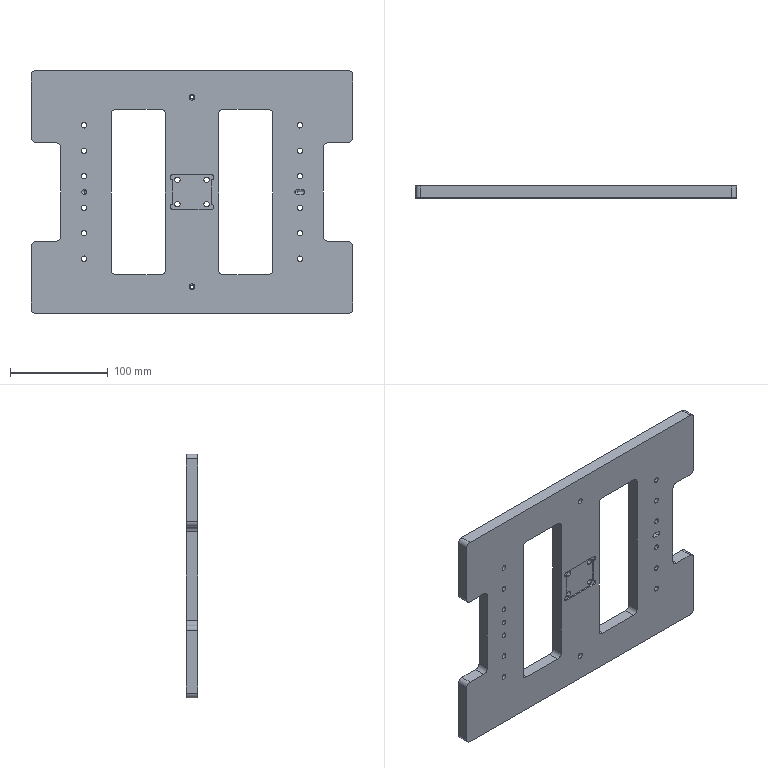Part | SolidWorks | features HoleWzd 5, ICE 4, Fillet 3, Extrusion 1 | 1 solid | 160 faces | box 329 x 12 x 250 mm | volume 676996 mm3 | cylinder 105 | plane 51 | cone 4 | commonest cylinder face diameters 10 x52 5.5 x32 5 x9 3.4 x4 6 x4 9.95 x4